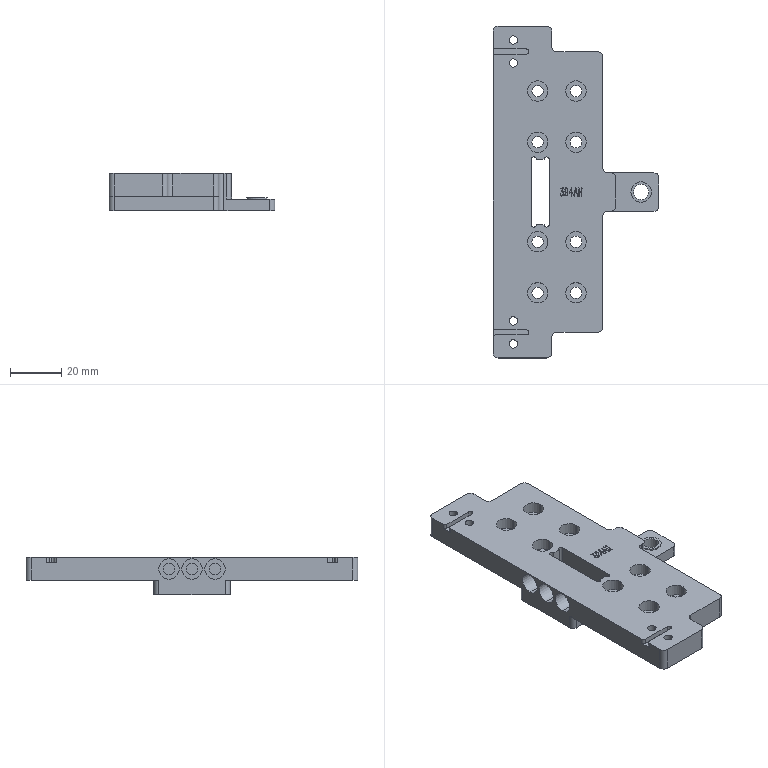NC program | NX | posted with a generic post | part box 65 x 130 x 14.5 mm
Lines 1 to 2036 of 11541:
N10 G17 G21 G94 G90
(ZLEVEL_PROFILE_1 , TOOL : D10)
N12 T15 M6
N14 G54
N16 G17 G0 G90 X-71.208 Y27.533 B0. C0. S9500 M3
N18 G43 Z30. H15
N20 Z5.5
N22 G94 G1 Z4.5 F1000.
N24 X-70.799 Y27.297
N26 G2 X-70.299 Y26.431 R1.
N28 G1 X-70.298 Y12.88 F2500.
N30 X-70.297 Y11.719
N32 X-70.3 Y11.5
N34 X-70.286 Y11.118
N36 G3 X-69.813 Y8.888 R8.291
N38 X-68.681 Y6.922 R8.266
N40 X-66.94 Y5.36 R8.297
N42 X-64.884 Y4.451 R8.318
N44 X-62.976 Y4.2 R9.828
N46 G1 X-60.3
N48 Y-8.884
N50 G3 X-54.907 Y-15.542 R7.364
N52 X-52.988 Y-15.8 R9.776
N54 G1 X-12.8
N56 Y-30.475
N58 X-12.787 Y-30.87
N60 G3 X-12.299 Y-33.146 R8.234
N62 X-11.168 Y-35.093 R8.428
N64 X-9.462 Y-36.627 R7.994
N66 X-7.381 Y-37.549 R8.218
N68 X-5.479 Y-37.8 R10.192
N70 G1 X5.633
N72 G3 X8.127 Y-37.307 R8.185
N74 X10.103 Y-36.16 R8.044
N76 X11.608 Y-34.491 R8.214
N78 X12.549 Y-32.384 R8.163
N80 X12.8 Y-30.475 R10.175
N82 G1 Y-15.8
N84 X13.005
N86 X52.98
N88 X53.391 Y-15.786
N90 G3 X55.595 Y-15.319 R8.354
N92 X57.599 Y-14.164 R8.095
N94 X59.12 Y-12.474 R8.359
N96 X60.044 Y-10.402 R8.156
N98 X60.3 Y-8.479 R9.732
N100 G1 Y4.2
N102 X63.167
N104 G3 X65.578 Y4.675 R8.47
N106 X67.604 Y5.839 R8.256
N108 X69.1 Y7.496 R8.528
N110 X70.054 Y9.635 R8.173
N112 X70.3 Y11.5 R9.88
N114 G1 X70.297 Y11.555
N116 X70.298 Y12.88
N118 X70.299 Y26.431
N120 G2 X70.799 Y27.297 R1.
N122 G1 X71.207 Y27.533
N124 Z5.5
N126 G0 Z30.
N128 X-71.208
N130 Z4.5
N132 G1 Z3.5 F1000.
N134 X-70.799 Y27.297
N136 G2 X-70.299 Y26.431 R1.
N138 G1 X-70.298 Y12.88 F2500.
N140 X-70.297 Y11.719
N142 X-70.3 Y11.5
N144 X-70.286 Y11.118
N146 G3 X-69.813 Y8.888 R8.275
N148 X-68.681 Y6.922 R8.238
N150 X-66.94 Y5.36 R8.281
N152 X-64.884 Y4.451 R8.265
N154 X-62.976 Y4.2 R9.757
N156 G1 X-60.3
N158 Y-8.863
N160 G3 X-54.907 Y-15.542 R7.358
N162 X-52.988 Y-15.8 R9.706
N164 G1 X-12.8
N166 Y-30.475
N168 X-12.787 Y-30.87
N170 G3 X-12.299 Y-33.146 R8.21
N172 X-11.168 Y-35.093 R8.408
N174 X-9.462 Y-36.627 R7.971
N176 X-7.381 Y-37.549 R8.21
N178 X-5.479 Y-37.8 R10.133
N180 G1 X5.629
N182 G3 X8.127 Y-37.307 R8.157
N184 X10.103 Y-36.16 R8.035
N186 X11.608 Y-34.491 R8.193
N188 X12.549 Y-32.384 R8.135
N190 X12.8 Y-30.475 R10.115
N192 G1 Y-15.8
N194 X13.005
N196 X52.98
N198 X53.391 Y-15.786
N200 G3 X55.595 Y-15.319 R8.337
N202 X57.599 Y-14.164 R8.073
N204 X59.12 Y-12.474 R8.337
N206 X60.044 Y-10.402 R8.14
N208 X60.3 Y-8.479 R9.662
N210 G1 Y4.2
N212 X63.165
N214 G3 X65.578 Y4.675 R8.441
N216 X67.604 Y5.839 R8.233
N218 X69.1 Y7.496 R8.511
N220 X70.054 Y9.635 R8.157
N222 X70.3 Y11.5 R9.803
N224 G1 X70.298 Y12.88
N226 X70.299 Y26.431
N228 G2 X70.799 Y27.297 R1.
N230 G1 X71.207 Y27.533
N232 Z4.5
N234 G0 Z30.
N236 X-71.208
N238 Z3.5
N240 G1 Z2.5 F1000.
N242 X-70.799 Y27.297
N244 G2 X-70.299 Y26.431 R1.
N246 G1 X-70.298 Y12.88 F2500.
N248 X-70.297 Y11.719
N250 X-70.3 Y11.5
N252 X-70.286 Y11.118
N254 G3 X-69.813 Y8.888 R8.225
N256 X-68.681 Y6.922 R8.211
N258 X-66.94 Y5.36 R8.264
N260 X-64.884 Y4.451 R8.247
N262 X-62.976 Y4.2 R9.687
N264 G1 X-60.3
N266 Y-8.863
N268 G3 X-54.907 Y-15.542 R7.358
N270 X-52.988 Y-15.8 R9.637
N272 G1 X-12.8
N274 Y-30.475
N276 X-12.787 Y-30.87
N278 G3 X-12.299 Y-33.146 R8.186
N280 X-11.168 Y-35.093 R8.388
N282 X-9.462 Y-36.627 R7.947
N284 X-7.381 Y-37.549 R8.196
N286 X-5.479 Y-37.8 R10.075
N288 G1 X5.625
N290 G3 X8.127 Y-37.307 R8.128
N292 X10.103 Y-36.16 R8.027
N294 X11.608 Y-34.491 R8.172
N296 X12.549 Y-32.384 R8.108
N298 X12.8 Y-30.475 R10.056
N300 G1 Y-15.8
N302 X13.005
N304 X52.98
N306 X53.391 Y-15.786
N308 G3 X55.595 Y-15.319 R8.32
N310 X57.599 Y-14.164 R8.051
N312 X59.12 Y-12.474 R8.314
N314 X60.044 Y-10.402 R8.123
N316 X60.3 Y-8.479 R9.593
N318 G1 Y4.2
N320 X63.162
N322 G3 X65.578 Y4.675 R8.412
N324 X67.604 Y5.839 R8.211
N326 X69.1 Y7.496 R8.49
N328 X70.054 Y9.635 R8.141
N330 X70.3 Y11.5 R9.727
N332 G1 X70.298 Y12.88
N334 X70.299 Y26.431
N336 G2 X70.799 Y27.297 R1.
N338 G1 X71.207 Y27.533
N340 Z3.5
N342 G0 Z30.
N344 X-71.208
N346 Z2.5
N348 G1 Z1.5 F1000.
N350 X-70.799 Y27.297
N352 G2 X-70.299 Y26.431 R1.
N354 G1 Y12.88 F2500.
N356 X-70.298 Y11.719
N358 X-70.3 Y11.5
N360 X-70.286 Y11.118
N362 G3 X-69.813 Y8.888 R8.208
N364 X-68.681 Y6.922 R8.184
N366 X-66.94 Y5.36 R8.247
N368 X-64.884 Y4.451 R8.23
N370 X-62.976 Y4.2 R9.619
N372 G1 X-60.3
N374 Y-8.862
N376 G3 X-54.907 Y-15.542 R7.358
N378 X-52.988 Y-15.8 R9.568
N380 G1 X-12.8
N382 Y-30.475
N384 X-12.787 Y-30.87
N386 G3 X-12.299 Y-33.146 R8.163
N388 X-11.168 Y-35.093 R8.368
N390 X-9.462 Y-36.627 R7.925
N392 X-7.381 Y-37.549 R8.173
N394 X-5.479 Y-37.8 R10.018
N396 G1 X5.62
N398 G3 X8.127 Y-37.307 R8.1
N400 X10.103 Y-36.16 R8.018
N402 X11.608 Y-34.491 R8.152
N404 X12.549 Y-32.384 R8.114
N406 X12.8 Y-30.475 R9.998
N408 G1 Y-15.8
N410 X13.005
N412 X52.98
N414 X53.391 Y-15.786
N416 G3 X55.595 Y-15.319 R8.304
N418 X57.599 Y-14.164 R8.03
N420 X59.12 Y-12.474 R8.292
N422 X60.044 Y-10.402 R8.104
N424 X60.3 Y-8.479 R9.526
N426 G1 Y4.2
N428 X63.159
N430 G3 X65.578 Y4.675 R8.378
N432 X67.604 Y5.839 R8.189
N434 X69.1 Y7.496 R8.462
N436 X70.054 Y9.635 R8.133
N438 X70.3 Y11.5 R9.652
N440 G1 X70.298 Y12.88
N442 X70.299 Y26.431
N444 G2 X70.799 Y27.297 R1.
N446 G1 X71.207 Y27.533
N448 Z2.5
N450 G0 Z30.
N452 X-71.208
N454 Z1.5
N456 G1 Z0.5 F1000.
N458 X-70.799 Y27.297
N460 G2 X-70.299 Y26.431 R1.
N462 G1 Y12.88 F2500.
N464 X-70.298 Y11.719
N466 X-70.3 Y11.5
N468 X-70.286 Y11.118
N470 G3 X-69.813 Y8.888 R8.189
N472 X-68.681 Y6.922 R8.158
N474 X-66.94 Y5.36 R8.231
N476 X-64.884 Y4.451 R8.212
N478 X-62.976 Y4.2 R9.551
N480 G1 X-60.3
N482 Y-8.852
N484 G3 X-54.907 Y-15.542 R7.355
N486 X-52.988 Y-15.8 R9.501
N488 G1 X-12.8
N490 Y-30.475
N492 X-12.787 Y-30.87
N494 G3 X-12.299 Y-33.146 R8.139
N496 X-11.168 Y-35.093 R8.348
N498 X-9.462 Y-36.627 R7.902
N500 X-7.381 Y-37.549 R8.15
N502 X-5.479 Y-37.8 R9.961
N504 G1 X5.615
N506 G3 X8.127 Y-37.307 R8.071
N508 X10.103 Y-36.16 R8.01
N510 X11.608 Y-34.491 R8.131
N512 X12.549 Y-32.384 R8.087
N514 X12.8 Y-30.475 R9.94
N516 G1 Y-15.8
N518 X13.005
N520 X52.98
N522 X53.391 Y-15.786
N524 G3 X55.595 Y-15.319 R8.287
N526 X57.599 Y-14.164 R8.008
N528 X59.12 Y-12.474 R8.269
N530 X60.044 Y-10.402 R8.084
N532 X60.3 Y-8.479 R9.459
N534 G1 Y4.2
N536 X63.155
N538 G3 X65.578 Y4.675 R8.345
N540 X67.604 Y5.839 R8.167
N542 X69.1 Y7.496 R8.435
N544 X70.054 Y9.635 R8.115
N546 X70.3 Y11.5 R9.579
N548 G1 X70.298 Y12.88
N550 X70.299 Y26.431
N552 G2 X70.799 Y27.297 R1.
N554 G1 X71.207 Y27.533
N556 Z1.5
N558 G0 Z30.
N560 X-71.208
N562 Z0.5
N564 G1 Z-0.5 F1000.
N566 X-70.799 Y27.297
N568 G2 X-70.299 Y26.431 R1.
N570 G1 Y12.88 F2500.
N572 X-70.3 Y11.5
N574 X-70.286 Y11.118
N576 G3 X-69.813 Y8.888 R8.17
N578 X-68.681 Y6.922 R8.131
N580 X-66.94 Y5.36 R8.215
N582 X-64.884 Y4.451 R8.189
N584 X-62.976 Y4.2 R9.484
N586 G1 X-60.3
N588 Y-8.859
N590 G3 X-54.907 Y-15.542 R7.357
N592 X-52.988 Y-15.8 R9.435
N594 G1 X-12.8
N596 Y-30.5
N598 G3 X-5.5 Y-37.8 R7.3
N600 G1 X5.5
N602 G3 X12.8 Y-30.5 R7.3
N604 G1 Y-15.8
N606 X52.98
N608 X53.391 Y-15.786
N610 G3 X55.595 Y-15.319 R8.271
N612 X57.599 Y-14.164 R7.987
N614 X59.12 Y-12.474 R8.247
N616 X60.044 Y-10.402 R8.065
N618 X60.3 Y-8.479 R9.393
N620 G1 Y4.2
N622 X63.152
N624 G3 X65.578 Y4.675 R8.312
N626 X67.604 Y5.839 R8.146
N628 X69.1 Y7.496 R8.401
N630 X70.054 Y9.635 R8.097
N632 X70.3 Y11.5 R9.507
N634 G1 X70.299 Y12.88
N636 Y26.431
N638 G2 X70.799 Y27.297 R1.
N640 G1 X71.207 Y27.533
N642 Z0.5
N644 G0 Z30.
N646 M5
(FLOOR_WALL_COPY_COPY , TOOL : D80)
N648 T19 M6
N650 G54
N652 G17 G0 G90 X-110. Y0. B0. C0. S6500 M3
N654 G43 Z30. H19
N656 Z7.04
N658 G94 G1 Z4.04 F1500.
N660 X-105.
N662 X105.
N664 X110.
N666 Z7.04
N668 G0 Z30.
N670 X-110.
N672 Z6.08
N674 G1 Z3.08
N676 X-105.
N678 X105.
N680 X110.
N682 Z6.08
N684 G0 Z30.
N686 X-110.
N688 Z5.12
N690 G1 Z2.12
N692 X-105.
N694 X105.
N696 X110.
N698 Z5.12
N700 G0 Z30.
N702 X-110.
N704 Z4.16
N706 G1 Z1.16
N708 X-105.
N710 X105.
N712 X110.
N714 Z4.16
N716 G0 Z30.
N718 X-110.
N720 Z3.2
N722 G1 Z0.2
N724 X-105.
N726 X105.
N728 X110.
N730 Z3.2
N732 G0 Z30.
(FLOOR_WALL_COPY_COPY_COPY , TOOL : D80)
N734 X-110.
N736 Z3.
N738 G1 Z0.
N740 X-105.
N742 X105.
N744 X110.
N746 Z3.
N748 G0 Z30.
N750 M5
(CAVITY_MILL_COPY_1 , TOOL : D10)
N752 T15 M6
N754 G54
N756 G17 G0 G90 X36.349 Y37.56 B0. C0. S9500 M3
N758 G43 Z30. H15
N760 Z0.1
N762 G94 G1 Z-0.9 F700.
N764 X38.947 Y33.06
N766 G3 X39.813 Y32.56 R1.
N768 G1 X58.06 F2500.
N770 X62.406
N772 X63.48 Y32.521
N774 X63.5 Y32.517
N776 X63.884 Y32.361
N778 X63.972 Y32.316
N780 X64.018 Y32.315
N782 X64.005 Y32.271
N784 G2 X64.765 Y31.516 R1.545
N786 G1 X64.785 Y31.48
N788 G2 X65.06 Y29.908 R2.587
N790 G1 X65.059 Y11.432
N792 X64.984 Y10.862
N794 X64.978 Y10.842
N796 X64.763 Y10.436
N798 X64.423 Y9.976
N800 X64.407 Y9.961
N802 X63.968 Y9.682
N804 X63.416 Y9.454
N806 X63.393 Y9.45
N808 X62.404 Y9.44
N810 X56.528
N812 X55.875 Y9.08
N814 X55.686 Y8.927
N816 X55.517 Y8.751
N818 X55.063 Y8.046
N820 X55.06 Y-3.562
N822 X55.058 Y-8.581
N824 X54.98 Y-9.154
N826 X54.973 Y-9.174
N828 X54.747 Y-9.59
N830 X54.405 Y-10.04
N832 X54.389 Y-10.055
N834 X53.775 Y-10.438
N836 X53.754 Y-10.446
N838 X53.159 Y-10.554
N840 X52.388 Y-10.56
N842 X38.521
N844 X37.905
N846 X37.751
N848 X19.859
N850 G2 X13.282 Y-15.656 R7.169
N852 G1 X13.218 Y-15.661
N854 X13.22 Y-15.597
N856 X13.257 Y-15.595
N858 G3 X20.1 Y-8.5 R7.1
N860 G1 Y30.5
N862 G3 X14.203 Y37.497 R7.1
N864 G1 X14.518
N866 G2 X19.859 Y32.56 R7.172
N868 G1 X39.813
N870 Y25.56
N872 X58.06
N874 X58.059 Y16.44
N876 X56.528
N878 G3 X53.149 Y15.571 R7.
N880 G1 X51.951 Y14.911
N882 X50.934 Y14.086
N884 X49.996 Y13.105
N886 X49.179 Y11.837
N888 G3 X48.063 Y8.048 R7.
N890 G1 X48.06 Y-3.56
N892 X38.519
N894 X27.1
N896 Y25.56
N898 X39.813
N900 Y18.56
N902 X45.527
N904 X50.825 Y20.299
N906 X45.527 Y18.56
N908 X44.474 Y17.46
N910 X43.294 Y15.629
N912 G3 X41.063 Y8.05 R14.
N914 G1 X41.062 Y3.44
N916 X34.1
N918 Y18.56
N920 X39.813
N922 G3 X40.679 Y19.06 R1.
N924 G1 Z0.1
N926 X36.349 Y37.56 Z-0.8 F5000.
N928 Z-1.8 F700.
N930 X38.947 Y33.06
N932 G3 X39.813 Y32.56 R1.
N934 G1 X58.06 F2500.
N936 X62.406
N938 X63.48 Y32.521
N940 X63.5 Y32.517
N942 X63.884 Y32.361
N944 X63.972 Y32.316
N946 X64.018 Y32.315
N948 X64.005 Y32.271
N950 G2 X64.765 Y31.516 R1.545
N952 G1 X64.785 Y31.48
N954 G2 X65.06 Y29.908 R2.587
N956 G1 X65.059 Y11.432
N958 X64.984 Y10.862
N960 X64.978 Y10.842
N962 X64.763 Y10.436
N964 X64.423 Y9.976
N966 X64.407 Y9.961
N968 X63.968 Y9.682
N970 X63.416 Y9.454
N972 X63.393 Y9.45
N974 X62.404 Y9.44
N976 X56.528
N978 X55.875 Y9.08
N980 X55.686 Y8.927
N982 X55.517 Y8.751
N984 X55.063 Y8.046
N986 X55.06 Y-3.562
N988 X55.058 Y-8.581
N990 X54.98 Y-9.154
N992 X54.973 Y-9.174
N994 X54.747 Y-9.59
N996 X54.405 Y-10.04
N998 X54.389 Y-10.055
N1000 X53.775 Y-10.438
N1002 X53.754 Y-10.446
N1004 X53.159 Y-10.554
N1006 X52.388 Y-10.56
N1008 X38.521
N1010 X37.905
N1012 X37.751
N1014 X19.859
N1016 G2 X13.282 Y-15.656 R7.169
N1018 G1 X13.218 Y-15.662
N1020 X13.22 Y-15.597
N1022 X13.257 Y-15.595
N1024 G3 X20.1 Y-8.5 R7.1
N1026 G1 Y30.5
N1028 G3 X14.202 Y37.497 R7.1
N1030 G1 X14.518
N1032 G2 X19.712 Y32.997 R7.172
N1034 X19.859 Y32.56 R7.172
N1036 G1 X39.813
N1038 Y25.56
N1040 X58.06
N1042 X58.059 Y16.44
N1044 X56.528
N1046 G3 X53.149 Y15.571 R7.
N1048 G1 X51.951 Y14.911
N1050 X50.934 Y14.086
N1052 X49.996 Y13.105
N1054 X49.179 Y11.837
N1056 G3 X48.063 Y8.048 R7.
N1058 G1 X48.06 Y-3.56
N1060 X38.519
N1062 X27.1
N1064 Y25.56
N1066 X39.813
N1068 Y18.56
N1070 X45.527
N1072 X50.825 Y20.299
N1074 X45.527 Y18.56
N1076 X44.474 Y17.46
N1078 X43.294 Y15.629
N1080 G3 X41.063 Y8.05 R14.
N1082 G1 X41.062 Y3.44
N1084 X34.1
N1086 Y18.56
N1088 X39.813
N1090 G3 X40.679 Y19.06 R1.
N1092 G1 Z-0.8
N1094 X36.349 Y37.56 Z-1.7 F5000.
N1096 Z-2.7 F700.
N1098 X38.947 Y33.06
N1100 G3 X39.813 Y32.56 R1.
N1102 G1 X58.06 F2500.
N1104 X62.406
N1106 X63.48 Y32.521
N1108 X63.5 Y32.517
N1110 X63.884 Y32.361
N1112 X63.972 Y32.316
N1114 X64.018 Y32.315
N1116 X64.005 Y32.271
N1118 G2 X64.765 Y31.516 R1.545
N1120 G1 X64.785 Y31.48
N1122 G2 X65.06 Y29.908 R2.587
N1124 G1 X65.059 Y11.432
N1126 X64.984 Y10.862
N1128 X64.978 Y10.842
N1130 X64.763 Y10.436
N1132 X64.423 Y9.976
N1134 X64.407 Y9.961
N1136 X63.968 Y9.682
N1138 X63.416 Y9.454
N1140 X63.393 Y9.45
N1142 X62.404 Y9.44
N1144 X56.528
N1146 X55.875 Y9.08
N1148 X55.686 Y8.927
N1150 X55.517 Y8.751
N1152 X55.063 Y8.046
N1154 X55.06 Y-3.562
N1156 X55.058 Y-8.581
N1158 X54.98 Y-9.154
N1160 X54.973 Y-9.174
N1162 X54.747 Y-9.59
N1164 X54.405 Y-10.04
N1166 X54.389 Y-10.055
N1168 X53.775 Y-10.438
N1170 X53.754 Y-10.446
N1172 X53.159 Y-10.554
N1174 X52.388 Y-10.56
N1176 X38.521
N1178 X37.905
N1180 X37.751
N1182 X19.859
N1184 G2 X13.282 Y-15.656 R7.169
N1186 G1 X13.218 Y-15.661
N1188 X13.22 Y-15.597
N1190 X13.257 Y-15.595
N1192 G3 X20.1 Y-8.5 R7.1
N1194 G1 Y30.5
N1196 G3 X14.201 Y37.498 R7.1
N1198 G1 X14.517
N1200 G2 X19.859 Y32.56 R7.172
N1202 G1 X39.813
N1204 Y25.56
N1206 X58.06
N1208 X58.059 Y16.44
N1210 X56.528
N1212 G3 X53.149 Y15.571 R7.
N1214 G1 X51.951 Y14.911
N1216 X50.934 Y14.086
N1218 X49.996 Y13.105
N1220 X49.179 Y11.837
N1222 G3 X48.063 Y8.048 R7.
N1224 G1 X48.06 Y-3.56
N1226 X38.519
N1228 X27.1
N1230 Y25.56
N1232 X39.813
N1234 Y18.56
N1236 X45.527
N1238 X50.825 Y20.299
N1240 X45.527 Y18.56
N1242 X44.474 Y17.46
N1244 X43.294 Y15.629
N1246 G3 X41.063 Y8.05 R14.
N1248 G1 X41.062 Y3.44
N1250 X34.1
N1252 Y18.56
N1254 X39.813
N1256 G3 X40.679 Y19.06 R1.
N1258 G1 Z-1.7
N1260 X36.349 Y37.56 Z-2.6 F5000.
N1262 Z-3.6 F700.
N1264 X38.947 Y33.06
N1266 G3 X39.813 Y32.56 R1.
N1268 G1 X58.06 F2500.
N1270 X62.406
N1272 X63.48 Y32.521
N1274 X63.5 Y32.517
N1276 X63.884 Y32.361
N1278 X63.972 Y32.316
N1280 X64.018 Y32.315
N1282 X64.005 Y32.271
N1284 G2 X64.765 Y31.516 R1.545
N1286 G1 X64.785 Y31.48
N1288 G2 X65.06 Y29.908 R2.587
N1290 G1 X65.059 Y11.432
N1292 X64.984 Y10.862
N1294 X64.978 Y10.842
N1296 X64.763 Y10.436
N1298 X64.423 Y9.976
N1300 X64.407 Y9.961
N1302 X63.968 Y9.682
N1304 X63.416 Y9.454
N1306 X63.393 Y9.45
N1308 X62.404 Y9.44
N1310 X56.528
N1312 X55.875 Y9.08
N1314 X55.686 Y8.927
N1316 X55.517 Y8.751
N1318 X55.063 Y8.046
N1320 X55.06 Y-3.562
N1322 X55.058 Y-8.581
N1324 X54.98 Y-9.154
N1326 X54.973 Y-9.174
N1328 X54.747 Y-9.59
N1330 X54.405 Y-10.04
N1332 X54.389 Y-10.055
N1334 X53.775 Y-10.438
N1336 X53.754 Y-10.446
N1338 X53.159 Y-10.554
N1340 X52.388 Y-10.56
N1342 X38.521
N1344 X37.905
N1346 X37.751
N1348 X19.859
N1350 G2 X13.282 Y-15.656 R7.169
N1352 G1 X13.218 Y-15.662
N1354 X13.22 Y-15.597
N1356 X13.257 Y-15.595
N1358 G3 X20.1 Y-8.5 R7.1
N1360 G1 Y30.5
N1362 G3 X14.2 Y37.498 R7.1
N1364 G1 X14.516
N1366 G2 X19.712 Y32.998 R7.172
N1368 X19.859 Y32.56 R7.172
N1370 G1 X39.813
N1372 Y25.56
N1374 X58.06
N1376 X58.059 Y16.44
N1378 X56.528
N1380 G3 X53.149 Y15.571 R7.
N1382 G1 X51.951 Y14.911
N1384 X50.934 Y14.086
N1386 X49.996 Y13.105
N1388 X49.179 Y11.837
N1390 G3 X48.063 Y8.048 R7.
N1392 G1 X48.06 Y-3.56
N1394 X38.519
N1396 X27.1
N1398 Y25.56
N1400 X39.813
N1402 Y18.56
N1404 X45.527
N1406 X50.825 Y20.299
N1408 X45.527 Y18.56
N1410 X44.474 Y17.46
N1412 X43.294 Y15.629
N1414 G3 X41.063 Y8.05 R14.
N1416 G1 X41.062 Y3.44
N1418 X34.1
N1420 Y18.56
N1422 X39.813
N1424 G3 X40.679 Y19.06 R1.
N1426 G1 Z-2.6
N1428 X36.349 Y37.56 Z-3.5 F5000.
N1430 Z-4.5 F700.
N1432 X38.947 Y33.06
N1434 G3 X39.813 Y32.56 R1.
N1436 G1 X58.06 F2500.
N1438 X62.406
N1440 X63.48 Y32.521
N1442 X63.5 Y32.517
N1444 X63.884 Y32.361
N1446 X63.972 Y32.316
N1448 X64.018 Y32.315
N1450 X64.005 Y32.271
N1452 G2 X64.765 Y31.516 R1.545
N1454 G1 X64.785 Y31.48
N1456 G2 X65.06 Y29.908 R2.587
N1458 G1 X65.059 Y11.432
N1460 X64.984 Y10.862
N1462 X64.978 Y10.842
N1464 X64.763 Y10.436
N1466 X64.423 Y9.976
N1468 X64.407 Y9.961
N1470 X63.968 Y9.682
N1472 X63.416 Y9.454
N1474 X63.393 Y9.45
N1476 X62.404 Y9.44
N1478 X56.528
N1480 X55.875 Y9.08
N1482 X55.686 Y8.927
N1484 X55.517 Y8.751
N1486 X55.063 Y8.046
N1488 X55.06 Y-3.562
N1490 X55.058 Y-8.581
N1492 X54.98 Y-9.154
N1494 X54.973 Y-9.174
N1496 X54.747 Y-9.59
N1498 X54.405 Y-10.04
N1500 X54.389 Y-10.055
N1502 X53.775 Y-10.438
N1504 X53.754 Y-10.446
N1506 X53.159 Y-10.554
N1508 X52.388 Y-10.56
N1510 X38.521
N1512 X37.905
N1514 X37.751
N1516 X19.859
N1518 G2 X13.282 Y-15.656 R7.169
N1520 G1 X13.218 Y-15.661
N1522 X13.22 Y-15.597
N1524 X13.257 Y-15.595
N1526 G3 X20.1 Y-8.5 R7.1
N1528 G1 Y30.5
N1530 G3 X14.199 Y37.498 R7.1
N1532 G1 X14.515
N1534 G2 X19.711 Y32.998 R7.172
N1536 X19.859 Y32.56 R7.172
N1538 G1 X39.813
N1540 Y25.56
N1542 X58.06
N1544 X58.059 Y16.44
N1546 X56.528
N1548 G3 X53.149 Y15.571 R7.
N1550 G1 X51.951 Y14.911
N1552 X50.934 Y14.086
N1554 X49.996 Y13.105
N1556 X49.179 Y11.837
N1558 G3 X48.063 Y8.048 R7.
N1560 G1 X48.06 Y-3.56
N1562 X38.519
N1564 X27.1
N1566 Y25.56
N1568 X39.813
N1570 Y18.56
N1572 X45.527
N1574 X50.825 Y20.299
N1576 X45.527 Y18.56
N1578 X44.474 Y17.46
N1580 X43.294 Y15.629
N1582 G3 X41.063 Y8.05 R14.
N1584 G1 X41.062 Y3.44
N1586 X34.1
N1588 Y18.56
N1590 X39.813
N1592 G3 X40.679 Y19.06 R1.
N1594 G1 Z-3.5
N1596 X36.349 Y37.56 Z-4.4 F5000.
N1598 Z-5.4 F700.
N1600 X38.947 Y33.06
N1602 G3 X39.813 Y32.56 R1.
N1604 G1 X58.06 F2500.
N1606 X62.406
N1608 X63.48 Y32.521
N1610 X63.5 Y32.517
N1612 X63.884 Y32.361
N1614 X63.972 Y32.316
N1616 X64.018 Y32.315
N1618 X64.005 Y32.271
N1620 G2 X64.765 Y31.516 R1.545
N1622 G1 X64.785 Y31.48
N1624 G2 X65.06 Y29.908 R2.587
N1626 G1 X65.059 Y11.432
N1628 X64.984 Y10.862
N1630 X64.978 Y10.842
N1632 X64.763 Y10.436
N1634 X64.423 Y9.976
N1636 X64.407 Y9.961
N1638 X63.968 Y9.682
N1640 X63.416 Y9.454
N1642 X63.393 Y9.45
N1644 X62.404 Y9.44
N1646 X56.528
N1648 X55.875 Y9.08
N1650 X55.686 Y8.927
N1652 X55.517 Y8.751
N1654 X55.063 Y8.046
N1656 X55.06 Y-3.562
N1658 X55.058 Y-8.581
N1660 X54.98 Y-9.154
N1662 X54.973 Y-9.174
N1664 X54.747 Y-9.59
N1666 X54.405 Y-10.04
N1668 X54.389 Y-10.055
N1670 X53.775 Y-10.438
N1672 X53.754 Y-10.446
N1674 X53.159 Y-10.554
N1676 X52.388 Y-10.56
N1678 X38.521
N1680 X37.905
N1682 X37.751
N1684 X19.859
N1686 G2 X13.282 Y-15.656 R7.169
N1688 G1 X13.218 Y-15.661
N1690 X13.22 Y-15.597
N1692 X13.257 Y-15.595
N1694 G3 X20.1 Y-8.5 R7.1
N1696 G1 Y30.5
N1698 G3 X14.198 Y37.498 R7.1
N1700 G1 X14.514
N1702 G2 X19.859 Y32.56 R7.172
N1704 G1 X39.813
N1706 Y25.56
N1708 X58.06
N1710 X58.059 Y16.44
N1712 X56.528
N1714 G3 X53.149 Y15.571 R7.
N1716 G1 X51.951 Y14.911
N1718 X50.934 Y14.086
N1720 X49.996 Y13.105
N1722 X49.179 Y11.837
N1724 G3 X48.063 Y8.048 R7.
N1726 G1 X48.06 Y-3.56
N1728 X38.519
N1730 X27.1
N1732 Y25.56
N1734 X39.813
N1736 Y18.56
N1738 X45.527
N1740 X50.825 Y20.299
N1742 X45.527 Y18.56
N1744 X44.474 Y17.46
N1746 X43.294 Y15.629
N1748 G3 X41.063 Y8.05 R14.
N1750 G1 X41.062 Y3.44
N1752 X34.1
N1754 Y18.56
N1756 X39.813
N1758 G3 X40.679 Y19.06 R1.
N1760 G1 Z-4.4
N1762 X35.842 Y-10.56 F5000.
N1764 X29. Z-6.233 F700.
N1766 X19.859 F2500.
N1768 G2 X13.282 Y-15.656 R7.169
N1770 G1 X13.218 Y-15.661
N1772 X13.22 Y-15.597
N1774 X13.257 Y-15.595
N1776 G3 X20.1 Y-8.5 R7.1
N1778 G1 Y25.4
N1780 X37.9
N1782 Y-10.56
N1784 X37.751
N1786 X29.
N1788 Y-3.56
N1790 X27.1
N1792 Y18.4
N1794 X30.9
N1796 Y-3.56
N1798 X29.
N1800 G3 X28.134 Y-4.06 R1.
N1802 G1 Z-5.233
N1804 X35.842 Y-10.56 F5000.
N1806 X29. Z-7.067 F700.
N1808 X19.859 F2500.
N1810 G2 X13.282 Y-15.656 R7.169
N1812 G1 X13.218 Y-15.661
N1814 X13.22 Y-15.597
N1816 X13.257 Y-15.595
N1818 G3 X20.1 Y-8.5 R7.1
N1820 G1 Y25.4
N1822 X37.9
N1824 Y-10.56
N1826 X37.751
N1828 X29.
N1830 Y-3.56
N1832 X27.1
N1834 Y18.4
N1836 X30.9
N1838 Y-3.56
N1840 X29.
N1842 G3 X28.134 Y-4.06 R1.
N1844 G1 Z-6.067
N1846 X35.842 Y-10.56 F5000.
N1848 X29. Z-7.9 F700.
N1850 X19.859 F2500.
N1852 G2 X13.282 Y-15.656 R7.169
N1854 G1 X13.218 Y-15.661
N1856 X13.22 Y-15.597
N1858 X13.257 Y-15.595
N1860 G3 X20.1 Y-8.5 R7.1
N1862 G1 Y25.4
N1864 X37.9
N1866 Y-10.56
N1868 X37.751
N1870 X29.
N1872 Y-3.56
N1874 X27.1
N1876 Y18.4
N1878 X30.9
N1880 Y-3.56
N1882 X29.
N1884 G3 X28.134 Y-4.06 R1.
N1886 G1 Z-6.9
N1888 G0 Z30.
N1890 X-43.246 Y37.56
N1892 Z0.1
N1894 G1 Z-0.9 F700.
N1896 X-40.648 Y33.06
N1898 G3 X-39.782 Y32.56 R1.
N1900 G1 X-19.859 F2500.
N1902 G2 X-14.498 Y37.497 R7.214
N1904 G1 X-14.203
N1906 G3 X-20.1 Y30.5 R7.1
N1908 G1 Y-8.5
N1910 G3 X-13.204 Y-15.597 R7.1
N1912 G1 Y-15.599
N1914 X-13.203 Y-15.662
N1916 X-13.267 Y-15.656
N1918 G2 X-19.859 Y-10.56 R7.166
N1920 G1 X-37.751
N1922 X-37.9
N1924 X-38.521
N1926 X-48.06
N1928 X-52.389
N1930 X-53.579 Y-10.55
N1932 X-53.61 Y-10.541
N1934 X-54.389 Y-10.055
N1936 X-54.405 Y-10.04
N1938 X-54.753 Y-9.582
N1940 X-54.973 Y-9.174
N1942 X-54.98 Y-9.154
N1944 X-55.059 Y-8.573
N1946 X-55.063 Y8.046
N1948 X-55.65 Y8.956
N1950 X-56.428 Y9.385
N1952 X-57.014 Y9.44
N1954 X-58.059
N1956 X-62.405
N1958 X-63.592 Y9.452
N1960 X-63.624 Y9.461
N1962 X-64.407 Y9.961
N1964 X-64.423 Y9.976
N1966 X-64.768 Y10.443
N1968 X-64.978 Y10.842
N1970 X-64.984 Y10.862
N1972 X-65.059 Y11.439
N1974 X-65.06 Y29.908
N1976 G2 X-64.769 Y31.511 R2.588
N1978 X-63.984 Y32.283 R1.577
N1980 G1 X-63.957 Y32.318
N1982 X-63.936 Y32.335
N1984 X-63.88 Y32.363
N1986 X-63.5 Y32.517
N1988 X-63.48 Y32.521
N1990 X-62.404 Y32.56
N1992 X-39.782
N1994 Y25.56
N1996 X-27.1
N1998 Y-3.56
N2000 X-48.06
N2002 X-48.063 Y8.048
N2004 G3 X-49.179 Y11.837 R7.
N2006 G1 X-49.765 Y12.747
N2008 G3 X-52.271 Y15.087 R7.
N2010 G1 X-53.05 Y15.516
N2012 G3 X-55.776 Y16.355 R7.
N2014 G1 X-56.687 Y16.44
N2016 X-58.059
N2018 X-58.06 Y25.56
N2020 X-39.782
N2022 Y18.56
N2024 X-34.1
N2026 Y3.44
N2028 X-41.062
N2030 X-41.063 Y8.05
N2032 G3 X-43.294 Y15.629 R14.
N2034 G1 X-43.881 Y16.539
N2036 G3 X-45.463 Y18.56 R14.
N2038 G1 X-50.795 Y20.29
N2040 X-45.463 Y18.56
N2042 X-39.782
N2044 G3 X-38.916 Y19.06 R1.
N2046 G1 Z0.1
N2048 X-43.246 Y37.56 Z-0.8 F5000.
N2050 Z-1.8 F700.
N2052 X-40.648 Y33.06
N2054 G3 X-39.782 Y32.56 R1.
N2056 G1 X-19.859 F2500.
N2058 G2 X-19.71 Y32.997 R7.214
N2060 X-14.497 Y37.497 R7.214
N2062 G1 X-14.202
N2064 G3 X-20.1 Y30.5 R7.1
N2066 G1 Y-8.5
N2068 G3 X-13.204 Y-15.597 R7.1
N2070 G1 X-13.208 Y-15.617
N2072 X-13.214 Y-15.671
N2074 X-13.267 Y-15.656
N2076 G2 X-19.859 Y-10.56 R7.166
N2078 G1 X-37.751
N2080 X-37.9
N2082 X-38.521
N2084 X-48.06
N2086 X-52.389
N2088 X-53.579 Y-10.55
N2090 X-53.61 Y-10.541
N2092 X-54.389 Y-10.055
N2094 X-54.405 Y-10.04
N2096 X-54.753 Y-9.582
N2098 X-54.973 Y-9.174
N2100 X-54.98 Y-9.154
N2102 X-55.059 Y-8.573
N2104 X-55.063 Y8.046
N2106 X-55.65 Y8.956
N2108 X-56.428 Y9.385
N2110 X-57.014 Y9.44
N2112 X-58.059
N2114 X-62.405
N2116 X-63.592 Y9.452
N2118 X-63.624 Y9.461
N2120 X-64.407 Y9.961
N2122 X-64.423 Y9.976
N2124 X-64.768 Y10.443
N2126 X-64.978 Y10.842
N2128 X-64.984 Y10.862
N2130 X-65.059 Y11.439
N2132 X-65.06 Y29.908
N2134 G2 X-64.769 Y31.511 R2.588
N2136 X-63.984 Y32.283 R1.577
N2138 G1 X-63.957 Y32.318
N2140 X-63.936 Y32.335
N2142 X-63.88 Y32.363
N2144 X-63.5 Y32.517
N2146 X-63.48 Y32.521
N2148 X-62.404 Y32.56
N2150 X-39.782
N2152 Y25.56
N2154 X-27.1
N2156 Y-3.56
N2158 X-48.06
N2160 X-48.063 Y8.048
N2162 G3 X-49.179 Y11.837 R7.
N2164 G1 X-49.765 Y12.747
N2166 G3 X-52.271 Y15.087 R7.
N2168 G1 X-53.05 Y15.516
N2170 G3 X-55.776 Y16.355 R7.
N2172 G1 X-56.687 Y16.44
N2174 X-58.059
N2176 X-58.06 Y25.56
N2178 X-39.782
N2180 Y18.56
N2182 X-34.1
N2184 Y3.44
N2186 X-41.062
N2188 X-41.063 Y8.05
N2190 G3 X-43.294 Y15.629 R14.
N2192 G1 X-43.881 Y16.539
N2194 G3 X-45.463 Y18.56 R14.
N2196 G1 X-50.795 Y20.29
N2198 X-45.463 Y18.56
N2200 X-39.782
N2202 G3 X-38.916 Y19.06 R1.
N2204 G1 Z-0.8
N2206 X-43.246 Y37.56 Z-1.7 F5000.
N2208 Z-2.7 F700.
N2210 X-40.648 Y33.06
N2212 G3 X-39.782 Y32.56 R1.
N2214 G1 X-19.859 F2500.
N2216 G2 X-14.496 Y37.498 R7.214
N2218 G1 X-14.201
N2220 G3 X-20.1 Y30.5 R7.1
N2222 G1 Y-8.5
N2224 G3 X-13.204 Y-15.597 R7.1
N2226 G1 X-13.203 Y-15.662
N2228 X-13.267 Y-15.656
N2230 G2 X-19.859 Y-10.56 R7.166
N2232 G1 X-37.751
N2234 X-37.9
N2236 X-38.521
N2238 X-48.06
N2240 X-52.389
N2242 X-53.579 Y-10.55
N2244 X-53.61 Y-10.541
N2246 X-54.389 Y-10.055
N2248 X-54.405 Y-10.04
N2250 X-54.753 Y-9.582
N2252 X-54.973 Y-9.174
N2254 X-54.98 Y-9.154
N2256 X-55.059 Y-8.573
N2258 X-55.063 Y8.046
N2260 X-55.65 Y8.956
N2262 X-56.428 Y9.385
N2264 X-57.014 Y9.44
N2266 X-58.059
N2268 X-62.405
N2270 X-63.592 Y9.452
N2272 X-63.624 Y9.461
N2274 X-64.407 Y9.961
N2276 X-64.423 Y9.976
N2278 X-64.768 Y10.443
N2280 X-64.978 Y10.842
N2282 X-64.984 Y10.862
N2284 X-65.059 Y11.439
N2286 X-65.06 Y29.908
N2288 G2 X-64.769 Y31.511 R2.588
N2290 X-63.984 Y32.283 R1.577
N2292 G1 X-63.957 Y32.318
N2294 X-63.936 Y32.335
N2296 X-63.88 Y32.363
N2298 X-63.5 Y32.517
N2300 X-63.48 Y32.521
N2302 X-62.404 Y32.56
N2304 X-39.782
N2306 Y25.56
N2308 X-27.1
N2310 Y-3.56
N2312 X-48.06
N2314 X-48.063 Y8.048
N2316 G3 X-49.179 Y11.837 R7.
N2318 G1 X-49.765 Y12.747
N2320 G3 X-52.271 Y15.087 R7.
N2322 G1 X-53.05 Y15.516
N2324 G3 X-55.776 Y16.355 R7.
N2326 G1 X-56.687 Y16.44
N2328 X-58.059
N2330 X-58.06 Y25.56
N2332 X-39.782
N2334 Y18.56
N2336 X-34.1
N2338 Y3.44
N2340 X-41.062
N2342 X-41.063 Y8.05
N2344 G3 X-43.294 Y15.629 R14.
N2346 G1 X-43.881 Y16.539
N2348 G3 X-45.463 Y18.56 R14.
N2350 G1 X-50.795 Y20.29
N2352 X-45.463 Y18.56
N2354 X-39.782
N2356 G3 X-38.916 Y19.06 R1.
N2358 G1 Z-1.7
N2360 X-43.246 Y37.56 Z-2.6 F5000.
N2362 Z-3.6 F700.
N2364 X-40.648 Y33.06
N2366 G3 X-39.782 Y32.56 R1.
N2368 G1 X-19.859 F2500.
N2370 G2 X-19.709 Y32.998 R7.214
N2372 X-14.495 Y37.498 R7.214
N2374 G1 X-14.2
N2376 G3 X-20.1 Y30.5 R7.1
N2378 G1 Y-8.501
N2380 G3 X-13.204 Y-15.597 R7.1
N2382 G1 Y-15.598
N2384 X-13.203 Y-15.662
N2386 X-13.267 Y-15.656
N2388 G2 X-19.859 Y-10.56 R7.166
N2390 G1 X-37.751
N2392 X-37.9
N2394 X-38.521
N2396 X-48.06
N2398 X-52.389
N2400 X-53.579 Y-10.55
N2402 X-53.61 Y-10.541
N2404 X-54.389 Y-10.055
N2406 X-54.405 Y-10.04
N2408 X-54.753 Y-9.582
N2410 X-54.973 Y-9.174
N2412 X-54.98 Y-9.154
N2414 X-55.059 Y-8.573
N2416 X-55.063 Y8.046
N2418 X-55.65 Y8.956
N2420 X-56.428 Y9.385
N2422 X-57.014 Y9.44
N2424 X-58.059
N2426 X-62.405
N2428 X-63.592 Y9.452
N2430 X-63.624 Y9.461
N2432 X-64.407 Y9.961
N2434 X-64.423 Y9.976
N2436 X-64.768 Y10.443
N2438 X-64.978 Y10.842
N2440 X-64.984 Y10.862
N2442 X-65.059 Y11.439
N2444 X-65.06 Y29.908
N2446 G2 X-64.769 Y31.511 R2.588
N2448 X-63.984 Y32.283 R1.577
N2450 G1 X-63.957 Y32.318
N2452 X-63.936 Y32.335
N2454 X-63.88 Y32.363
N2456 X-63.5 Y32.517
N2458 X-63.48 Y32.521
N2460 X-62.404 Y32.56
N2462 X-39.782
N2464 Y25.56
N2466 X-27.1
N2468 Y-3.56
N2470 X-48.06
N2472 X-48.063 Y8.048
N2474 G3 X-49.179 Y11.837 R7.
N2476 G1 X-49.765 Y12.747
N2478 G3 X-52.271 Y15.087 R7.
N2480 G1 X-53.05 Y15.516
N2482 G3 X-55.776 Y16.355 R7.
N2484 G1 X-56.687 Y16.44
N2486 X-58.059
N2488 X-58.06 Y25.56
N2490 X-39.782
N2492 Y18.56
N2494 X-34.1
N2496 Y3.44
N2498 X-41.062
N2500 X-41.063 Y8.05
N2502 G3 X-43.294 Y15.629 R14.
N2504 G1 X-43.881 Y16.539
N2506 G3 X-45.463 Y18.56 R14.
N2508 G1 X-50.795 Y20.29
N2510 X-45.463 Y18.56
N2512 X-39.782
N2514 G3 X-38.916 Y19.06 R1.
N2516 G1 Z-2.6
N2518 X-43.246 Y37.56 Z-3.5 F5000.
N2520 Z-4.5 F700.
N2522 X-40.648 Y33.06
N2524 G3 X-39.782 Y32.56 R1.
N2526 G1 X-21.247 F2500.
N2528 X-19.859
N2530 G2 X-14.494 Y37.498 R7.214
N2532 G1 X-14.199
N2534 G3 X-20.1 Y30.5 R7.1
N2536 G1 Y-8.5
N2538 G3 X-19.42 Y-11.532 R7.1
N2540 X-13.204 Y-15.597 R7.1
N2542 G1 X-13.205 Y-15.602
N2544 Y-15.664
N2546 X-13.267 Y-15.656
N2548 G2 X-19.859 Y-10.56 R7.166
N2550 G1 X-37.751
N2552 X-37.9
N2554 X-38.521
N2556 X-48.06
N2558 X-52.389
N2560 X-53.579 Y-10.55
N2562 X-53.61 Y-10.541
N2564 X-54.389 Y-10.055
N2566 X-54.405 Y-10.04
N2568 X-54.753 Y-9.582
N2570 X-54.973 Y-9.174
N2572 X-54.98 Y-9.154
N2574 X-55.059 Y-8.573
N2576 X-55.063 Y8.046
N2578 X-55.65 Y8.956
N2580 X-56.428 Y9.385
N2582 X-57.014 Y9.44
N2584 X-58.059
N2586 X-62.405
N2588 X-63.592 Y9.452
N2590 X-63.624 Y9.461
N2592 X-64.407 Y9.961
N2594 X-64.423 Y9.976
N2596 X-64.768 Y10.443
N2598 X-64.978 Y10.842
N2600 X-64.984 Y10.862
N2602 X-65.059 Y11.439
N2604 X-65.06 Y29.908
N2606 G2 X-64.769 Y31.511 R2.588
N2608 X-63.984 Y32.283 R1.577
N2610 G1 X-63.957 Y32.318
N2612 X-63.936 Y32.335
N2614 X-63.88 Y32.363
N2616 X-63.5 Y32.517
N2618 X-63.48 Y32.521
N2620 X-62.404 Y32.56
N2622 X-39.782
N2624 Y25.56
N2626 X-27.1
N2628 Y-3.56
N2630 X-48.06
N2632 X-48.063 Y8.048
N2634 G3 X-49.179 Y11.837 R7.
N2636 G1 X-49.765 Y12.747
N2638 G3 X-52.271 Y15.087 R7.
N2640 G1 X-53.05 Y15.516
N2642 G3 X-55.776 Y16.355 R7.
N2644 G1 X-56.687 Y16.44
N2646 X-58.059
N2648 X-58.06 Y25.56
N2650 X-39.782
N2652 Y18.56
N2654 X-34.1
N2656 Y3.44
N2658 X-41.062
N2660 X-41.063 Y8.05
N2662 G3 X-43.294 Y15.629 R14.
N2664 G1 X-43.881 Y16.539
N2666 G3 X-45.463 Y18.56 R14.
N2668 G1 X-50.795 Y20.29
N2670 X-45.463 Y18.56
N2672 X-39.782
N2674 G3 X-38.916 Y19.06 R1.
N2676 G1 Z-3.5
N2678 X-43.246 Y37.56 Z-4.4 F5000.
N2680 Z-5.4 F700.
N2682 X-40.648 Y33.06
N2684 G3 X-39.782 Y32.56 R1.
N2686 G1 X-19.859 F2500.
N2688 G2 X-14.494 Y37.498 R7.214
N2690 G1 X-14.198
N2692 G3 X-20.1 Y30.5 R7.1
N2694 G1 Y-8.5
N2696 G3 X-13.204 Y-15.597 R7.1
N2698 G1 Y-15.599
N2700 X-13.203 Y-15.662
N2702 X-13.267 Y-15.656
N2704 G2 X-19.859 Y-10.56 R7.166
N2706 G1 X-37.751
N2708 X-37.9
N2710 X-38.521
N2712 X-48.06
N2714 X-52.389
N2716 X-53.579 Y-10.55
N2718 X-53.61 Y-10.541
N2720 X-54.389 Y-10.055
N2722 X-54.405 Y-10.04
N2724 X-54.753 Y-9.582
N2726 X-54.973 Y-9.174
N2728 X-54.98 Y-9.154
N2730 X-55.059 Y-8.573
N2732 X-55.063 Y8.046
N2734 X-55.65 Y8.956
N2736 X-56.428 Y9.385
N2738 X-57.014 Y9.44
N2740 X-58.059
N2742 X-62.405
N2744 X-63.592 Y9.452
N2746 X-63.624 Y9.461
N2748 X-64.407 Y9.961
N2750 X-64.423 Y9.976
N2752 X-64.768 Y10.443
N2754 X-64.978 Y10.842
N2756 X-64.984 Y10.862
N2758 X-65.059 Y11.439
N2760 X-65.06 Y29.908
N2762 G2 X-64.769 Y31.511 R2.588
N2764 X-63.984 Y32.283 R1.577
N2766 G1 X-63.957 Y32.318
N2768 X-63.936 Y32.335
N2770 X-63.88 Y32.363
N2772 X-63.5 Y32.517
N2774 X-63.48 Y32.521
N2776 X-62.404 Y32.56
N2778 X-39.782
N2780 Y25.56
N2782 X-27.1
N2784 Y-3.56
N2786 X-48.06
N2788 X-48.063 Y8.048
N2790 G3 X-49.179 Y11.837 R7.
N2792 G1 X-49.765 Y12.747
N2794 G3 X-52.271 Y15.087 R7.
N2796 G1 X-53.05 Y15.516
N2798 G3 X-55.776 Y16.355 R7.
N2800 G1 X-56.687 Y16.44
N2802 X-58.059
N2804 X-58.06 Y25.56
N2806 X-39.782
N2808 Y18.56
N2810 X-34.1
N2812 Y3.44
N2814 X-41.062
N2816 X-41.063 Y8.05
N2818 G3 X-43.294 Y15.629 R14.
N2820 G1 X-43.881 Y16.539
N2822 G3 X-45.463 Y18.56 R14.
N2824 G1 X-50.795 Y20.29
N2826 X-45.463 Y18.56
N2828 X-39.782
N2830 G3 X-38.916 Y19.06 R1.
N2832 G1 Z-4.4
N2834 X-22.158 Y-10.56 F5000.
N2836 X-29. Z-6.233 F700.
N2838 X-37.751 F2500.
N2840 X-37.9
N2842 Y-3.56
N2844 Y25.4
N2846 X-20.1
N2848 Y-8.5
N2850 G3 X-13.204 Y-15.597 R7.1
N2852 G1 Y-15.598
N2854 X-13.203 Y-15.662
N2856 X-13.267 Y-15.656
N2858 G2 X-19.859 Y-10.56 R7.166
N2860 G1 X-29.
N2862 Y-3.56
N2864 X-30.9
N2866 Y18.4
N2868 X-27.1
N2870 Y-3.56
N2872 X-29.
N2874 G3 X-29.866 Y-4.06 R1.
N2876 G1 Z-5.233
N2878 X-22.158 Y-10.56 F5000.
N2880 X-29. Z-7.067 F700.
N2882 X-37.751 F2500.
N2884 X-37.9
N2886 Y-3.56
N2888 Y25.4
N2890 X-20.1
N2892 Y-8.5
N2894 G3 X-13.204 Y-15.597 R7.1
N2896 G1 Y-15.598
N2898 X-13.203 Y-15.662
N2900 X-13.267 Y-15.656
N2902 G2 X-19.859 Y-10.56 R7.166
N2904 G1 X-29.
N2906 Y-3.56
N2908 X-30.9
N2910 Y18.4
N2912 X-27.1
N2914 Y-3.56
N2916 X-29.
N2918 G3 X-29.866 Y-4.06 R1.
N2920 G1 Z-6.067
N2922 X-22.158 Y-10.56 F5000.
N2924 X-29. Z-7.9 F700.
N2926 X-37.751 F2500.
N2928 X-37.9
N2930 Y-3.56
N2932 Y25.4
N2934 X-20.1
N2936 Y-8.5
N2938 G3 X-13.204 Y-15.597 R7.1
N2940 G1 Y-15.598
N2942 X-13.203 Y-15.662
N2944 X-13.267 Y-15.656
N2946 G2 X-19.859 Y-10.56 R7.166
N2948 G1 X-29.
N2950 Y-3.56
N2952 X-30.9
N2954 Y18.4
N2956 X-27.1
N2958 Y-3.56
N2960 X-29.
N2962 G3 X-29.866 Y-4.06 R1.
N2964 G1 Z-6.9
N2966 G0 Z30.
N2968 M5
(CAVITY_MILL_COPY_1_COPY , TOOL : D4)
N2970 T11 M6
N2972 G54
N2974 G17 G0 G90 X40.2 Y24.564 B0. C0. S9500 M3
N2976 G43 Z30. H11
N2978 Z-4.857
N2980 G94 G1 Z-5.857 F700.
N2982 X40.5 Y24.737
N2984 G3 X41. Y25.603 R1.
N2986 G1 Y28.5 F1650.
N2988 X38.103
N2990 G3 X37.237 Y28. R1.
N2992 G1 X37.064 Y27.7
N2994 Z-4.857
N2996 G0 Z30.
N2998 X40.2 Y24.564
N3000 Z-5.214
N3002 G1 Z-6.214 F700.
N3004 X40.5 Y24.737
N3006 G3 X41. Y25.603 R1.
N3008 G1 Y28.5 F1650.
N3010 X38.103
N3012 G3 X37.237 Y28. R1.
N3014 G1 X37.064 Y27.7
N3016 Z-5.214
N3018 G0 X40.2 Y24.564 Z-5.571
N3020 G1 Z-6.571 F700.
N3022 X40.5 Y24.737
N3024 G3 X41. Y25.603 R1.
N3026 G1 Y28.5 F1650.
N3028 X38.103
N3030 G3 X37.237 Y28. R1.
N3032 G1 X37.064 Y27.7
N3034 Z-5.571
N3036 G0 X40.2 Y24.564 Z-5.929
N3038 G1 Z-6.929 F700.
N3040 X40.5 Y24.737
N3042 G3 X41. Y25.603 R1.
N3044 G1 Y28.5 F1650.
N3046 X38.103
N3048 G3 X37.237 Y28. R1.
N3050 G1 X37.064 Y27.7
N3052 Z-5.929
N3054 G0 X40.2 Y24.564 Z-6.286
N3056 G1 Z-7.286 F700.
N3058 X40.5 Y24.737
N3060 G3 X41. Y25.603 R1.
N3062 G1 Y28.5 F1650.
N3064 X38.103
N3066 G3 X37.237 Y28. R1.
N3068 G1 X37.064 Y27.7
N3070 Z-6.286
N3072 G0 X40.2 Y24.564 Z-6.643
N3074 G1 Z-7.643 F700.
N3076 X40.5 Y24.737
N3078 G3 X41. Y25.603 R1.
N3080 G1 Y28.5 F1650.
N3082 X38.103
N3084 G3 X37.237 Y28. R1.
N3086 G1 X37.064 Y27.7
N3088 Z-6.643
N3090 G0 X40.2 Y24.564 Z-7.
N3092 G1 Z-8. F700.
N3094 X40.5 Y24.737
N3096 G3 X41. Y25.603 R1.
N3098 G1 Y28.5 F1650.
N3100 X38.103
N3102 G3 X37.237 Y28. R1.
N3104 G1 X37.064 Y27.7
N3106 Z-7.
N3108 G0 Z30.
N3110 X20.936
N3112 Z-4.857
N3114 G1 Z-5.857 F700.
N3116 X20.763 Y28.
N3118 G3 X19.897 Y28.5 R1.
N3120 G1 X17. F1650.
N3122 Y25.603
N3124 G3 X17.5 Y24.737 R1.
N3126 G1 X17.8 Y24.564
N3128 Z-4.857
N3130 G0 Z30.
N3132 X20.936 Y27.7
N3134 Z-5.214
N3136 G1 Z-6.214 F700.
N3138 X20.763 Y28.
N3140 G3 X19.897 Y28.5 R1.
N3142 G1 X17. F1650.
N3144 Y25.603
N3146 G3 X17.5 Y24.737 R1.
N3148 G1 X17.8 Y24.564
N3150 Z-5.214
N3152 G0 X20.936 Y27.7 Z-5.571
N3154 G1 Z-6.571 F700.
N3156 X20.763 Y28.
N3158 G3 X19.897 Y28.5 R1.
N3160 G1 X17. F1650.
N3162 Y25.603
N3164 G3 X17.5 Y24.737 R1.
N3166 G1 X17.8 Y24.564
N3168 Z-5.571
N3170 G0 X20.936 Y27.7 Z-5.929
N3172 G1 Z-6.929 F700.
N3174 X20.763 Y28.
N3176 G3 X19.897 Y28.5 R1.
N3178 G1 X17. F1650.
N3180 Y25.603
N3182 G3 X17.5 Y24.737 R1.
N3184 G1 X17.8 Y24.564
N3186 Z-5.929
N3188 G0 X20.936 Y27.7 Z-6.286
N3190 G1 Z-7.286 F700.
N3192 X20.763 Y28.
N3194 G3 X19.897 Y28.5 R1.
N3196 G1 X17. F1650.
N3198 Y25.603
N3200 G3 X17.5 Y24.737 R1.
N3202 G1 X17.8 Y24.564
N3204 Z-6.286
N3206 G0 X20.936 Y27.7 Z-6.643
N3208 G1 Z-7.643 F700.
N3210 X20.763 Y28.
N3212 G3 X19.897 Y28.5 R1.
N3214 G1 X17. F1650.
N3216 Y25.603
N3218 G3 X17.5 Y24.737 R1.
N3220 G1 X17.8 Y24.564
N3222 Z-6.643
N3224 G0 X20.936 Y27.7 Z-7.
N3226 G1 Z-8. F700.
N3228 X20.763 Y28.
N3230 G3 X19.897 Y28.5 R1.
N3232 G1 X17. F1650.
N3234 Y25.603
N3236 G3 X17.5 Y24.737 R1.
N3238 G1 X17.8 Y24.564
N3240 Z-7.
N3242 G0 Z30.
N3244 X-17.8
N3246 Z-4.857
N3248 G1 Z-5.857 F700.
N3250 X-17.5 Y24.737
N3252 G3 X-17. Y25.603 R1.
N3254 G1 Y28.5 F1650.
N3256 X-19.897
N3258 G3 X-20.763 Y28. R1.
N3260 G1 X-20.936 Y27.7
N3262 Z-4.857
N3264 G0 Z30.
N3266 X-17.8 Y24.564
N3268 Z-5.214
N3270 G1 Z-6.214 F700.
N3272 X-17.5 Y24.737
N3274 G3 X-17. Y25.603 R1.
N3276 G1 Y28.5 F1650.
N3278 X-19.897
N3280 G3 X-20.763 Y28. R1.
N3282 G1 X-20.936 Y27.7
N3284 Z-5.214
N3286 G0 X-17.8 Y24.564 Z-5.571
N3288 G1 Z-6.571 F700.
N3290 X-17.5 Y24.737
N3292 G3 X-17. Y25.603 R1.
N3294 G1 Y28.5 F1650.
N3296 X-19.897
N3298 G3 X-20.763 Y28. R1.
N3300 G1 X-20.936 Y27.7
N3302 Z-5.571
N3304 G0 X-17.8 Y24.564 Z-5.929
N3306 G1 Z-6.929 F700.
N3308 X-17.5 Y24.737
N3310 G3 X-17. Y25.603 R1.
N3312 G1 Y28.5 F1650.
N3314 X-19.897
N3316 G3 X-20.763 Y28. R1.
N3318 G1 X-20.936 Y27.7
N3320 Z-5.929
N3322 G0 X-17.8 Y24.564 Z-6.286
N3324 G1 Z-7.286 F700.
N3326 X-17.5 Y24.737
N3328 G3 X-17. Y25.603 R1.
N3330 G1 Y28.5 F1650.
N3332 X-19.897
N3334 G3 X-20.763 Y28. R1.
N3336 G1 X-20.936 Y27.7
N3338 Z-6.286
N3340 G0 X-17.8 Y24.564 Z-6.643
N3342 G1 Z-7.643 F700.
N3344 X-17.5 Y24.737
N3346 G3 X-17. Y25.603 R1.
N3348 G1 Y28.5 F1650.
N3350 X-19.897
N3352 G3 X-20.763 Y28. R1.
N3354 G1 X-20.936 Y27.7
N3356 Z-6.643
N3358 G0 X-17.8 Y24.564 Z-7.
N3360 G1 Z-8. F700.
N3362 X-17.5 Y24.737
N3364 G3 X-17. Y25.603 R1.
N3366 G1 Y28.5 F1650.
N3368 X-19.897
N3370 G3 X-20.763 Y28. R1.
N3372 G1 X-20.936 Y27.7
N3374 Z-7.
N3376 G0 Z30.
N3378 X-37.064
N3380 Z-4.857
N3382 G1 Z-5.857 F700.
N3384 X-37.237 Y28.
N3386 G3 X-38.103 Y28.5 R1.
N3388 G1 X-41. F1650.
N3390 Y25.603
N3392 G3 X-40.5 Y24.737 R1.
N3394 G1 X-40.2 Y24.564
N3396 Z-4.857
N3398 G0 Z30.
N3400 X-37.064 Y27.7
N3402 Z-5.214
N3404 G1 Z-6.214 F700.
N3406 X-37.237 Y28.
N3408 G3 X-38.103 Y28.5 R1.
N3410 G1 X-41. F1650.
N3412 Y25.603
N3414 G3 X-40.5 Y24.737 R1.
N3416 G1 X-40.2 Y24.564
N3418 Z-5.214
N3420 G0 X-37.064 Y27.7 Z-5.571
N3422 G1 Z-6.571 F700.
N3424 X-37.237 Y28.
N3426 G3 X-38.103 Y28.5 R1.
N3428 G1 X-41. F1650.
N3430 Y25.603
N3432 G3 X-40.5 Y24.737 R1.
N3434 G1 X-40.2 Y24.564
N3436 Z-5.571
N3438 G0 X-37.064 Y27.7 Z-5.929
N3440 G1 Z-6.929 F700.
N3442 X-37.237 Y28.
N3444 G3 X-38.103 Y28.5 R1.
N3446 G1 X-41. Y28.499 F1650.
N3448 Y25.603
N3450 G3 X-40.5 Y24.737 R1.
N3452 G1 X-40.2 Y24.564
N3454 Z-5.929
N3456 G0 X-37.064 Y27.7 Z-6.286
N3458 G1 Z-7.286 F700.
N3460 X-37.237 Y28.
N3462 G3 X-38.103 Y28.5 R1.
N3464 G1 X-41. Y28.499 F1650.
N3466 Y25.603
N3468 G3 X-40.5 Y24.737 R1.
N3470 G1 X-40.2 Y24.564
N3472 Z-6.286
N3474 G0 X-37.064 Y27.7 Z-6.643
N3476 G1 Z-7.643 F700.
N3478 X-37.237 Y28.
N3480 G3 X-38.103 Y28.5 R1.
N3482 G1 X-41. Y28.499 F1650.
N3484 Y25.603
N3486 G3 X-40.5 Y24.737 R1.
N3488 G1 X-40.2 Y24.564
N3490 Z-6.643
N3492 G0 X-37.064 Y27.7 Z-7.
N3494 G1 Z-8. F700.
N3496 X-37.237 Y28.
N3498 G3 X-38.103 Y28.5 R1.
N3500 G1 X-41. Y28.499 F1650.
N3502 Y25.603
N3504 G3 X-40.5 Y24.737 R1.
N3506 G1 X-40.2 Y24.564
N3508 Z-7.
N3510 G0 Z30.
(FLOOR_WALL_COPY_1 , TOOL : D4)
N3512 X-70.424 Y10.437
N3514 Z-4.
N3516 G1 Z-5.5 F1250.
N3518 X-69.2 Y11.144
N3520 G3 X-69. Y11.49 R0.4
N3522 G1 Y30.51
N3524 G2 X-67.046 Y34.931 R6.
N3526 G1 Y7.069
N3528 G3 X-65.091 Y5.876 R6.
N3530 G1 Y36.124
N3532 G2 X-63.137 Y36.498 R6.
N3534 G1 Y5.502
N3536 X-63. Y5.5
N3538 X-61.183
N3540 Y36.5
N3542 X-59.229
N3544 Y5.5
N3546 X-59. Y-8.5
N3548 X-58.887 Y-9.659
N3550 X-58.552 Y-10.775
N3552 X-58.008 Y-11.805
N3554 X-57.274 Y-12.711
N3556 Y36.5
N3558 X-55.32
N3560 Y-14.033
N3562 G3 X-53.366 Y-14.489 R6.
N3564 G1 Y36.5
N3566 X-51.412
N3568 Y-14.5
N3570 X-49.457
N3572 Y36.5
N3574 X-47.503
N3576 Y-14.5
N3578 X-45.549
N3580 Y36.5
N3582 X-43.595
N3584 Y-14.5
N3586 X-41.64
N3588 Y36.5
N3590 X-39.686
N3592 Y-14.5
N3594 X-39.
N3596 X-37.732 Y26.5
N3598 Y36.5
N3600 X-35.778
N3602 Y26.5
N3604 X-33.823
N3606 Y36.5
N3608 X-31.869
N3610 Y26.5
N3612 X-29.915
N3614 Y36.5
N3616 X-27.96
N3618 Y26.5
N3620 X-26.006
N3622 Y36.5
N3624 X-24.052
N3626 Y26.5
N3628 X-22.098
N3630 Y36.5
N3632 X-20.143
N3634 Y26.5
N3636 X-19. Y25.5
N3638 X-18.189
N3640 Y36.5
N3642 X-16.235
N3644 Y33.179
N3646 G2 X-14.281 Y34.5 R4.2
N3648 G1 Y36.5
N3650 X-12.326
N3652 Y34.7
N3654 Z-4.
N3656 G0 Z30.
N3658 X-19.179 Y24.011
N3660 Z-4.
N3662 G1 Z-5.5
N3664 X-17.2 Y25.154
N3666 G3 X-17. Y25.5 R0.4
N3668 G1 Y30.5
N3670 G2 X-13. Y34.5 R4.
N3672 G1 X-9.
N3674 G3 X-8.654 Y34.7 R0.4
N3676 G1 X-7.511 Y36.679
N3678 Z-4.
N3680 G0 Z30.
N3682 X14.012 Y38.
N3684 Z-4.
N3686 G1 Z-5.5
N3688 Y34.796
N3690 G3 X14.281 Y34.5 R0.4
N3692 G1 Y36.5
N3694 X16.247
N3696 Y33.164
N3698 G2 X17.2 Y30.5 R4.2
N3700 G1 Y25.5
N3702 X18.213
N3704 Y36.5
N3706 X20.179
N3708 Y26.5
N3710 X22.145
N3712 Y36.5
N3714 X24.111
N3716 Y26.5
N3718 X26.077
N3720 Y36.5
N3722 X28.044
N3724 Y26.5
N3726 X30.01
N3728 Y36.5
N3730 X31.976
N3732 Y26.5
N3734 X33.942
N3736 Y36.5
N3738 X35.908
N3740 Y26.5
N3742 X37.874
N3744 Y36.5
N3746 X39.84
N3748 Y-14.5
N3750 X41.806
N3752 Y36.5
N3754 X43.773
N3756 Y-14.5
N3758 X45.739
N3760 Y36.5
N3762 X47.705
N3764 Y-14.5
N3766 X49.671
N3768 Y36.5
N3770 X51.637
N3772 Y-14.5
N3774 X53.
N3776 G3 X53.603 Y-14.47 R6.
N3778 G1 Y36.5
N3780 X55.569
N3782 Y-13.922
N3784 G3 X57.535 Y-12.428 R6.
N3786 G1 Y36.5
N3788 X59.502
N3790 Y5.5
N3792 X61.468
N3794 Y36.5
N3796 X63.
N3798 G2 X63.434 Y36.484 R6.
N3800 G1 Y5.516
N3802 G3 X65.4 Y6.001 R6.
N3804 G1 Y35.999
N3806 G3 X65.2 Y36.346 R0.4
N3808 G1 X65.642 Y37.519
N3810 Z-4.
N3812 G0 Z30.
N3814 X7.511 Y36.679
N3816 Z-4.
N3818 G1 Z-5.5
N3820 X8.654 Y34.7
N3822 G3 X9. Y34.5 R0.4
N3824 G1 X13.
N3826 G2 X17. Y30.5 R4.
N3828 G1 Y25.5
N3830 G3 X17.2 Y25.154 R0.4
N3832 G1 X19.179 Y24.011
N3834 Z-4.
N3836 G0 Z30.
(FLOOR_WALL_COPY_1_COPY , TOOL : D4)
N3838 X-14.462 Y-14.
N3840 Z-6.5
N3842 G1 Z-8.
N3844 X-14.576 Y-12.729
N3846 G3 X-14.807 Y-12.402 R0.4
N3848 G1 Y-12.5
N3850 X-16.798
N3852 Y-10.516
N3854 G2 X-17.3 Y-8.5 R4.3
N3856 G1 Y28.2
N3858 X-18.79
N3860 Y-12.5
N3862 X-20.782
N3864 Y28.2
N3866 X-22.774
N3868 Y-12.5
N3870 X-24.766
N3872 Y28.2
N3874 X-26.757
N3876 Y-12.5
N3878 X-28.749
N3880 Y28.2
N3882 X-30.741
N3884 Y-12.5
N3886 X-32.733
N3888 Y28.2
N3890 X-34.725
N3892 Y-12.5
N3894 X-36.716
N3896 Y28.2
N3898 X-38.708
N3900 Y-12.5
N3902 X-40.7
N3904 Y28.2
N3906 Z-6.5
N3908 G0 Z30.
N3910 X-13.367 Y-14.088
N3912 Z-6.5
N3914 G1 Z-8.
N3916 X-13.739 Y-12.75
N3918 G3 X-14.024 Y-12.47 R0.4
N3920 G2 X-17.1 Y-8.5 R4.1
N3922 G1 Y28.4
N3924 X-40.9
N3926 Y-12.5
N3928 G3 X-40.7 Y-12.846 R0.4
N3930 G1 X-38.702 Y-14.
N3932 Z-6.5
N3934 G0 Z30.
N3936 X12.435 Y-14.1
N3938 Z-6.5
N3940 G1 Z-8.
N3942 X14.607 Y-12.846
N3944 G3 X14.807 Y-12.5 R0.4
N3946 G1 Y-12.402
N3948 G3 X16.798 Y-10.516 R4.3
N3950 G1 Y-12.5
N3952 X18.79
N3954 Y28.2
N3956 X20.782
N3958 Y-12.5
N3960 X22.774
N3962 Y28.2
N3964 X24.766
N3966 Y-12.5
N3968 X26.757
N3970 Y28.2
N3972 X28.749
N3974 Y-12.5
N3976 X30.741
N3978 Y28.2
N3980 X32.733
N3982 Y-12.5
N3984 X34.725
N3986 Y28.2
N3988 X36.716
N3990 Y-12.5
N3992 X38.708
N3994 Y28.2
N3996 X40.7
N3998 Y-12.5
N4000 G2 X40.5 Y-12.846 R0.4
N4002 G1 X38.502 Y-14.
N4004 Z-6.5
N4006 G0 Z30.
N4008 X38.702
N4010 Z-6.5
N4012 G1 Z-8.
N4014 X40.7 Y-12.846
N4016 G3 X40.9 Y-12.5 R0.4
N4018 G1 Y28.4
N4020 X17.1
N4022 Y-8.5
N4024 G2 X14.024 Y-12.47 R4.1
N4026 G3 X13.739 Y-12.75 R0.4
N4028 G1 X13.367 Y-14.088
N4030 Z-6.5
N4032 G0 Z30.
N4034 M5